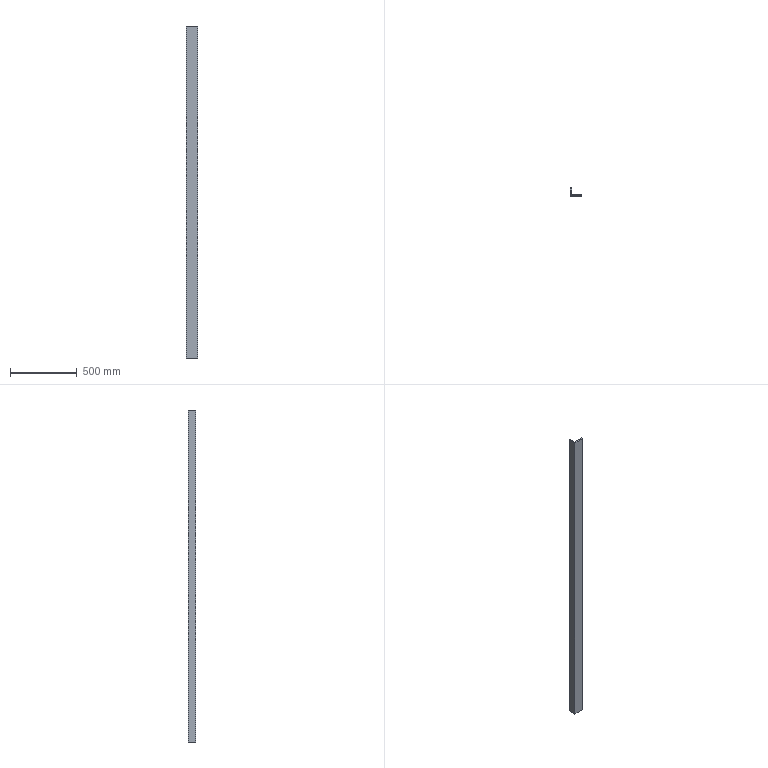Part | STEP file | Positioning angle steel_Default<As machined> | 1 solid | 8 faces | box 83 x 58 x 2484 mm | volume 2642976 mm3 | plane 8
STEP:
#1=CARTESIAN_POINT('',(0.,0.,0.));
#2=DIRECTION('',(0.,0.,1.));
#3=DIRECTION('',(1.,0.,0.));
#4=AXIS2_PLACEMENT_3D('',#1,#2,#3);
#5=CARTESIAN_POINT('',(2684.309,1399.529,5287.416));
#6=VERTEX_POINT('',#5);
#7=CARTESIAN_POINT('',(2684.309,1407.529,5287.416));
#8=VERTEX_POINT('',#7);
#9=CARTESIAN_POINT('',(2684.309,1399.529,5287.416));
#10=DIRECTION('',(0.,1.,0.));
#11=VECTOR('',#10,1.);
#12=LINE('',#9,#11);
#13=CARTESIAN_POINT('',(2684.309,1399.529,5388.673));
#14=DIRECTION('',(-1.,0.,0.));
#15=DIRECTION('',(0.,0.,1.));
#16=AXIS2_PLACEMENT_3D('',#13,#14,#15);
#17=PLANE('',#16);
#18=CARTESIAN_POINT('',(-101.257,0.));
#19=DIRECTION('',(0.,1.));
#20=VECTOR('',#19,1.);
#21=LINE('',#18,#20);
#22=(GEOMETRIC_REPRESENTATION_CONTEXT(2)PARAMETRIC_REPRESENTATION_CONTEXT()REPRESENTATION_CONTEXT('',''));
#23=DEFINITIONAL_REPRESENTATION('',(#21),#22);
#24=PCURVE('',#17,#23);
#25=CARTESIAN_POINT('',(1791.123,-1401.429,5287.416));
#26=DIRECTION('',(0.,0.,1.));
#27=DIRECTION('',(1.,0.,0.));
#28=AXIS2_PLACEMENT_3D('',#25,#26,#27);
#29=PLANE('',#28);
#30=CARTESIAN_POINT('',(893.186,2800.958));
#31=DIRECTION('',(0.,1.));
#32=VECTOR('',#31,1.);
#33=LINE('',#30,#32);
#34=(GEOMETRIC_REPRESENTATION_CONTEXT(2)PARAMETRIC_REPRESENTATION_CONTEXT()REPRESENTATION_CONTEXT('',''));
#35=DEFINITIONAL_REPRESENTATION('',(#33),#34);
#36=PCURVE('',#29,#35);
#37=SURFACE_CURVE('',#12,(#24,#36),.PCURVE_S1.);
#38=EDGE_CURVE('',#6,#8,#37,.T.);
#39=ORIENTED_EDGE('',*,*,#38,.F.);
#40=CARTESIAN_POINT('',(2684.309,1399.529,2803.416));
#41=VERTEX_POINT('',#40);
#42=CARTESIAN_POINT('',(2684.309,1399.529,5388.673));
#43=DIRECTION('',(0.,0.,-1.));
#44=VECTOR('',#43,1.);
#45=LINE('',#42,#44);
#46=CARTESIAN_POINT('',(0.,0.));
#47=DIRECTION('',(-1.,0.));
#48=VECTOR('',#47,1.);
#49=LINE('',#46,#48);
#50=(GEOMETRIC_REPRESENTATION_CONTEXT(2)PARAMETRIC_REPRESENTATION_CONTEXT()REPRESENTATION_CONTEXT('',''));
#51=DEFINITIONAL_REPRESENTATION('',(#49),#50);
#52=PCURVE('',#17,#51);
#53=CARTESIAN_POINT('',(2601.309,1399.529,5388.673));
#54=DIRECTION('',(0.,1.,0.));
#55=DIRECTION('',(0.,0.,1.));
#56=AXIS2_PLACEMENT_3D('',#53,#54,#55);
#57=PLANE('',#56);
#58=CARTESIAN_POINT('',(0.,83.));
#59=DIRECTION('',(-1.,0.));
#60=VECTOR('',#59,1.);
#61=LINE('',#58,#60);
#62=(GEOMETRIC_REPRESENTATION_CONTEXT(2)PARAMETRIC_REPRESENTATION_CONTEXT()REPRESENTATION_CONTEXT('',''));
#63=DEFINITIONAL_REPRESENTATION('',(#61),#62);
#64=PCURVE('',#57,#63);
#65=SURFACE_CURVE('',#45,(#52,#64),.PCURVE_S1.);
#66=EDGE_CURVE('',#6,#41,#65,.T.);
#67=ORIENTED_EDGE('',*,*,#66,.T.);
#68=CARTESIAN_POINT('',(2684.309,1407.529,2803.416));
#69=VERTEX_POINT('',#68);
#70=CARTESIAN_POINT('',(2684.309,1399.529,2803.416));
#71=DIRECTION('',(0.,1.,0.));
#72=VECTOR('',#71,1.);
#73=LINE('',#70,#72);
#74=CARTESIAN_POINT('',(-2585.257,0.));
#75=DIRECTION('',(0.,1.));
#76=VECTOR('',#75,1.);
#77=LINE('',#74,#76);
#78=(GEOMETRIC_REPRESENTATION_CONTEXT(2)PARAMETRIC_REPRESENTATION_CONTEXT()REPRESENTATION_CONTEXT('',''));
#79=DEFINITIONAL_REPRESENTATION('',(#77),#78);
#80=PCURVE('',#17,#79);
#81=CARTESIAN_POINT('',(0.,0.,2803.416));
#82=DIRECTION('',(0.,0.,1.));
#83=DIRECTION('',(1.,0.,0.));
#84=AXIS2_PLACEMENT_3D('',#81,#82,#83);
#85=PLANE('',#84);
#86=CARTESIAN_POINT('',(2684.309,1399.529));
#87=DIRECTION('',(0.,1.));
#88=VECTOR('',#87,1.);
#89=LINE('',#86,#88);
#90=(GEOMETRIC_REPRESENTATION_CONTEXT(2)PARAMETRIC_REPRESENTATION_CONTEXT()REPRESENTATION_CONTEXT('',''));
#91=DEFINITIONAL_REPRESENTATION('',(#89),#90);
#92=PCURVE('',#85,#91);
#93=SURFACE_CURVE('',#73,(#80,#92),.PCURVE_S1.);
#94=EDGE_CURVE('',#41,#69,#93,.T.);
#95=ORIENTED_EDGE('',*,*,#94,.T.);
#96=CARTESIAN_POINT('',(2684.309,1407.529,5388.673));
#97=DIRECTION('',(0.,0.,-1.));
#98=VECTOR('',#97,1.);
#99=LINE('',#96,#98);
#100=CARTESIAN_POINT('',(0.,8.));
#101=DIRECTION('',(-1.,0.));
#102=VECTOR('',#101,1.);
#103=LINE('',#100,#102);
#104=(GEOMETRIC_REPRESENTATION_CONTEXT(2)PARAMETRIC_REPRESENTATION_CONTEXT()REPRESENTATION_CONTEXT('',''));
#105=DEFINITIONAL_REPRESENTATION('',(#103),#104);
#106=PCURVE('',#17,#105);
#107=CARTESIAN_POINT('',(2684.309,1407.529,5388.673));
#108=DIRECTION('',(0.,-1.,0.));
#109=DIRECTION('',(0.,0.,-1.));
#110=AXIS2_PLACEMENT_3D('',#107,#108,#109);
#111=PLANE('',#110);
#112=CARTESIAN_POINT('',(0.,0.));
#113=DIRECTION('',(1.,0.));
#114=VECTOR('',#113,1.);
#115=LINE('',#112,#114);
#116=(GEOMETRIC_REPRESENTATION_CONTEXT(2)PARAMETRIC_REPRESENTATION_CONTEXT()REPRESENTATION_CONTEXT('',''));
#117=DEFINITIONAL_REPRESENTATION('',(#115),#116);
#118=PCURVE('',#111,#117);
#119=SURFACE_CURVE('',#99,(#106,#118),.PCURVE_S1.);
#120=EDGE_CURVE('',#8,#69,#119,.T.);
#121=ORIENTED_EDGE('',*,*,#120,.F.);
#122=EDGE_LOOP('',(#39,#67,#95,#121));
#123=FACE_BOUND('',#122,.T.);
#124=ADVANCED_FACE('',(#123),#17,.F.);
#125=CARTESIAN_POINT('',(2609.309,1407.529,5287.416));
#126=VERTEX_POINT('',#125);
#127=CARTESIAN_POINT('',(2684.309,1407.529,5287.416));
#128=DIRECTION('',(-1.,0.,0.));
#129=VECTOR('',#128,1.);
#130=LINE('',#127,#129);
#131=CARTESIAN_POINT('',(101.257,0.));
#132=DIRECTION('',(0.,-1.));
#133=VECTOR('',#132,1.);
#134=LINE('',#131,#133);
#135=(GEOMETRIC_REPRESENTATION_CONTEXT(2)PARAMETRIC_REPRESENTATION_CONTEXT()REPRESENTATION_CONTEXT('',''));
#136=DEFINITIONAL_REPRESENTATION('',(#134),#135);
#137=PCURVE('',#111,#136);
#138=CARTESIAN_POINT('',(893.186,2808.958));
#139=DIRECTION('',(-1.,0.));
#140=VECTOR('',#139,1.);
#141=LINE('',#138,#140);
#142=(GEOMETRIC_REPRESENTATION_CONTEXT(2)PARAMETRIC_REPRESENTATION_CONTEXT()REPRESENTATION_CONTEXT('',''));
#143=DEFINITIONAL_REPRESENTATION('',(#141),#142);
#144=PCURVE('',#29,#143);
#145=SURFACE_CURVE('',#130,(#137,#144),.PCURVE_S1.);
#146=EDGE_CURVE('',#8,#126,#145,.T.);
#147=ORIENTED_EDGE('',*,*,#146,.F.);
#148=ORIENTED_EDGE('',*,*,#120,.T.);
#149=CARTESIAN_POINT('',(2609.309,1407.529,2803.416));
#150=VERTEX_POINT('',#149);
#151=CARTESIAN_POINT('',(2684.309,1407.529,2803.416));
#152=DIRECTION('',(-1.,0.,0.));
#153=VECTOR('',#152,1.);
#154=LINE('',#151,#153);
#155=CARTESIAN_POINT('',(2585.257,0.));
#156=DIRECTION('',(0.,-1.));
#157=VECTOR('',#156,1.);
#158=LINE('',#155,#157);
#159=(GEOMETRIC_REPRESENTATION_CONTEXT(2)PARAMETRIC_REPRESENTATION_CONTEXT()REPRESENTATION_CONTEXT('',''));
#160=DEFINITIONAL_REPRESENTATION('',(#158),#159);
#161=PCURVE('',#111,#160);
#162=CARTESIAN_POINT('',(2684.309,1407.529));
#163=DIRECTION('',(-1.,0.));
#164=VECTOR('',#163,1.);
#165=LINE('',#162,#164);
#166=(GEOMETRIC_REPRESENTATION_CONTEXT(2)PARAMETRIC_REPRESENTATION_CONTEXT()REPRESENTATION_CONTEXT('',''));
#167=DEFINITIONAL_REPRESENTATION('',(#165),#166);
#168=PCURVE('',#85,#167);
#169=SURFACE_CURVE('',#154,(#161,#168),.PCURVE_S1.);
#170=EDGE_CURVE('',#69,#150,#169,.T.);
#171=ORIENTED_EDGE('',*,*,#170,.T.);
#172=CARTESIAN_POINT('',(2609.309,1407.529,5388.673));
#173=DIRECTION('',(0.,0.,-1.));
#174=VECTOR('',#173,1.);
#175=LINE('',#172,#174);
#176=CARTESIAN_POINT('',(0.,-75.));
#177=DIRECTION('',(1.,0.));
#178=VECTOR('',#177,1.);
#179=LINE('',#176,#178);
#180=(GEOMETRIC_REPRESENTATION_CONTEXT(2)PARAMETRIC_REPRESENTATION_CONTEXT()REPRESENTATION_CONTEXT('',''));
#181=DEFINITIONAL_REPRESENTATION('',(#179),#180);
#182=PCURVE('',#111,#181);
#183=CARTESIAN_POINT('',(2609.309,1407.529,5388.673));
#184=DIRECTION('',(-1.,0.,0.));
#185=DIRECTION('',(0.,0.,1.));
#186=AXIS2_PLACEMENT_3D('',#183,#184,#185);
#187=PLANE('',#186);
#188=CARTESIAN_POINT('',(0.,0.));
#189=DIRECTION('',(-1.,0.));
#190=VECTOR('',#189,1.);
#191=LINE('',#188,#190);
#192=(GEOMETRIC_REPRESENTATION_CONTEXT(2)PARAMETRIC_REPRESENTATION_CONTEXT()REPRESENTATION_CONTEXT('',''));
#193=DEFINITIONAL_REPRESENTATION('',(#191),#192);
#194=PCURVE('',#187,#193);
#195=SURFACE_CURVE('',#175,(#182,#194),.PCURVE_S1.);
#196=EDGE_CURVE('',#126,#150,#195,.T.);
#197=ORIENTED_EDGE('',*,*,#196,.F.);
#198=EDGE_LOOP('',(#147,#148,#171,#197));
#199=FACE_BOUND('',#198,.T.);
#200=ADVANCED_FACE('',(#199),#111,.F.);
#201=CARTESIAN_POINT('',(2609.309,1457.529,5287.416));
#202=VERTEX_POINT('',#201);
#203=CARTESIAN_POINT('',(2609.309,1407.529,5287.416));
#204=DIRECTION('',(0.,1.,0.));
#205=VECTOR('',#204,1.);
#206=LINE('',#203,#205);
#207=CARTESIAN_POINT('',(-101.257,0.));
#208=DIRECTION('',(0.,1.));
#209=VECTOR('',#208,1.);
#210=LINE('',#207,#209);
#211=(GEOMETRIC_REPRESENTATION_CONTEXT(2)PARAMETRIC_REPRESENTATION_CONTEXT()REPRESENTATION_CONTEXT('',''));
#212=DEFINITIONAL_REPRESENTATION('',(#210),#211);
#213=PCURVE('',#187,#212);
#214=CARTESIAN_POINT('',(818.186,2808.958));
#215=DIRECTION('',(0.,1.));
#216=VECTOR('',#215,1.);
#217=LINE('',#214,#216);
#218=(GEOMETRIC_REPRESENTATION_CONTEXT(2)PARAMETRIC_REPRESENTATION_CONTEXT()REPRESENTATION_CONTEXT('',''));
#219=DEFINITIONAL_REPRESENTATION('',(#217),#218);
#220=PCURVE('',#29,#219);
#221=SURFACE_CURVE('',#206,(#213,#220),.PCURVE_S1.);
#222=EDGE_CURVE('',#126,#202,#221,.T.);
#223=ORIENTED_EDGE('',*,*,#222,.F.);
#224=ORIENTED_EDGE('',*,*,#196,.T.);
#225=CARTESIAN_POINT('',(2609.309,1457.529,2803.416));
#226=VERTEX_POINT('',#225);
#227=CARTESIAN_POINT('',(2609.309,1407.529,2803.416));
#228=DIRECTION('',(0.,1.,0.));
#229=VECTOR('',#228,1.);
#230=LINE('',#227,#229);
#231=CARTESIAN_POINT('',(-2585.257,0.));
#232=DIRECTION('',(0.,1.));
#233=VECTOR('',#232,1.);
#234=LINE('',#231,#233);
#235=(GEOMETRIC_REPRESENTATION_CONTEXT(2)PARAMETRIC_REPRESENTATION_CONTEXT()REPRESENTATION_CONTEXT('',''));
#236=DEFINITIONAL_REPRESENTATION('',(#234),#235);
#237=PCURVE('',#187,#236);
#238=CARTESIAN_POINT('',(2609.309,1407.529));
#239=DIRECTION('',(0.,1.));
#240=VECTOR('',#239,1.);
#241=LINE('',#238,#240);
#242=(GEOMETRIC_REPRESENTATION_CONTEXT(2)PARAMETRIC_REPRESENTATION_CONTEXT()REPRESENTATION_CONTEXT('',''));
#243=DEFINITIONAL_REPRESENTATION('',(#241),#242);
#244=PCURVE('',#85,#243);
#245=SURFACE_CURVE('',#230,(#237,#244),.PCURVE_S1.);
#246=EDGE_CURVE('',#150,#226,#245,.T.);
#247=ORIENTED_EDGE('',*,*,#246,.T.);
#248=CARTESIAN_POINT('',(2609.309,1457.529,5388.673));
#249=DIRECTION('',(0.,0.,-1.));
#250=VECTOR('',#249,1.);
#251=LINE('',#248,#250);
#252=CARTESIAN_POINT('',(0.,50.));
#253=DIRECTION('',(-1.,0.));
#254=VECTOR('',#253,1.);
#255=LINE('',#252,#254);
#256=(GEOMETRIC_REPRESENTATION_CONTEXT(2)PARAMETRIC_REPRESENTATION_CONTEXT()REPRESENTATION_CONTEXT('',''));
#257=DEFINITIONAL_REPRESENTATION('',(#255),#256);
#258=PCURVE('',#187,#257);
#259=CARTESIAN_POINT('',(2609.309,1457.529,5388.673));
#260=DIRECTION('',(0.,-1.,0.));
#261=DIRECTION('',(0.,0.,-1.));
#262=AXIS2_PLACEMENT_3D('',#259,#260,#261);
#263=PLANE('',#262);
#264=CARTESIAN_POINT('',(0.,0.));
#265=DIRECTION('',(1.,0.));
#266=VECTOR('',#265,1.);
#267=LINE('',#264,#266);
#268=(GEOMETRIC_REPRESENTATION_CONTEXT(2)PARAMETRIC_REPRESENTATION_CONTEXT()REPRESENTATION_CONTEXT('',''));
#269=DEFINITIONAL_REPRESENTATION('',(#267),#268);
#270=PCURVE('',#263,#269);
#271=SURFACE_CURVE('',#251,(#258,#270),.PCURVE_S1.);
#272=EDGE_CURVE('',#202,#226,#271,.T.);
#273=ORIENTED_EDGE('',*,*,#272,.F.);
#274=EDGE_LOOP('',(#223,#224,#247,#273));
#275=FACE_BOUND('',#274,.T.);
#276=ADVANCED_FACE('',(#275),#187,.F.);
#277=CARTESIAN_POINT('',(2601.309,1457.529,5287.416));
#278=VERTEX_POINT('',#277);
#279=CARTESIAN_POINT('',(2609.309,1457.529,5287.416));
#280=DIRECTION('',(-1.,0.,0.));
#281=VECTOR('',#280,1.);
#282=LINE('',#279,#281);
#283=CARTESIAN_POINT('',(101.257,0.));
#284=DIRECTION('',(0.,-1.));
#285=VECTOR('',#284,1.);
#286=LINE('',#283,#285);
#287=(GEOMETRIC_REPRESENTATION_CONTEXT(2)PARAMETRIC_REPRESENTATION_CONTEXT()REPRESENTATION_CONTEXT('',''));
#288=DEFINITIONAL_REPRESENTATION('',(#286),#287);
#289=PCURVE('',#263,#288);
#290=CARTESIAN_POINT('',(818.186,2858.958));
#291=DIRECTION('',(-1.,0.));
#292=VECTOR('',#291,1.);
#293=LINE('',#290,#292);
#294=(GEOMETRIC_REPRESENTATION_CONTEXT(2)PARAMETRIC_REPRESENTATION_CONTEXT()REPRESENTATION_CONTEXT('',''));
#295=DEFINITIONAL_REPRESENTATION('',(#293),#294);
#296=PCURVE('',#29,#295);
#297=SURFACE_CURVE('',#282,(#289,#296),.PCURVE_S1.);
#298=EDGE_CURVE('',#202,#278,#297,.T.);
#299=ORIENTED_EDGE('',*,*,#298,.F.);
#300=ORIENTED_EDGE('',*,*,#272,.T.);
#301=CARTESIAN_POINT('',(2601.309,1457.529,2803.416));
#302=VERTEX_POINT('',#301);
#303=CARTESIAN_POINT('',(2609.309,1457.529,2803.416));
#304=DIRECTION('',(-1.,0.,0.));
#305=VECTOR('',#304,1.);
#306=LINE('',#303,#305);
#307=CARTESIAN_POINT('',(2585.257,0.));
#308=DIRECTION('',(0.,-1.));
#309=VECTOR('',#308,1.);
#310=LINE('',#307,#309);
#311=(GEOMETRIC_REPRESENTATION_CONTEXT(2)PARAMETRIC_REPRESENTATION_CONTEXT()REPRESENTATION_CONTEXT('',''));
#312=DEFINITIONAL_REPRESENTATION('',(#310),#311);
#313=PCURVE('',#263,#312);
#314=CARTESIAN_POINT('',(2609.309,1457.529));
#315=DIRECTION('',(-1.,0.));
#316=VECTOR('',#315,1.);
#317=LINE('',#314,#316);
#318=(GEOMETRIC_REPRESENTATION_CONTEXT(2)PARAMETRIC_REPRESENTATION_CONTEXT()REPRESENTATION_CONTEXT('',''));
#319=DEFINITIONAL_REPRESENTATION('',(#317),#318);
#320=PCURVE('',#85,#319);
#321=SURFACE_CURVE('',#306,(#313,#320),.PCURVE_S1.);
#322=EDGE_CURVE('',#226,#302,#321,.T.);
#323=ORIENTED_EDGE('',*,*,#322,.T.);
#324=CARTESIAN_POINT('',(2601.309,1457.529,5388.673));
#325=DIRECTION('',(0.,0.,-1.));
#326=VECTOR('',#325,1.);
#327=LINE('',#324,#326);
#328=CARTESIAN_POINT('',(0.,-8.));
#329=DIRECTION('',(1.,0.));
#330=VECTOR('',#329,1.);
#331=LINE('',#328,#330);
#332=(GEOMETRIC_REPRESENTATION_CONTEXT(2)PARAMETRIC_REPRESENTATION_CONTEXT()REPRESENTATION_CONTEXT('',''));
#333=DEFINITIONAL_REPRESENTATION('',(#331),#332);
#334=PCURVE('',#263,#333);
#335=CARTESIAN_POINT('',(2601.309,1457.529,5388.673));
#336=DIRECTION('',(1.,0.,0.));
#337=DIRECTION('',(0.,0.,-1.));
#338=AXIS2_PLACEMENT_3D('',#335,#336,#337);
#339=PLANE('',#338);
#340=CARTESIAN_POINT('',(0.,0.));
#341=DIRECTION('',(1.,0.));
#342=VECTOR('',#341,1.);
#343=LINE('',#340,#342);
#344=(GEOMETRIC_REPRESENTATION_CONTEXT(2)PARAMETRIC_REPRESENTATION_CONTEXT()REPRESENTATION_CONTEXT('',''));
#345=DEFINITIONAL_REPRESENTATION('',(#343),#344);
#346=PCURVE('',#339,#345);
#347=SURFACE_CURVE('',#327,(#334,#346),.PCURVE_S1.);
#348=EDGE_CURVE('',#278,#302,#347,.T.);
#349=ORIENTED_EDGE('',*,*,#348,.F.);
#350=EDGE_LOOP('',(#299,#300,#323,#349));
#351=FACE_BOUND('',#350,.T.);
#352=ADVANCED_FACE('',(#351),#263,.F.);
#353=CARTESIAN_POINT('',(2601.309,1399.529,5287.416));
#354=VERTEX_POINT('',#353);
#355=CARTESIAN_POINT('',(2601.309,1457.529,5287.416));
#356=DIRECTION('',(0.,-1.,0.));
#357=VECTOR('',#356,1.);
#358=LINE('',#355,#357);
#359=CARTESIAN_POINT('',(101.257,0.));
#360=DIRECTION('',(0.,-1.));
#361=VECTOR('',#360,1.);
#362=LINE('',#359,#361);
#363=(GEOMETRIC_REPRESENTATION_CONTEXT(2)PARAMETRIC_REPRESENTATION_CONTEXT()REPRESENTATION_CONTEXT('',''));
#364=DEFINITIONAL_REPRESENTATION('',(#362),#363);
#365=PCURVE('',#339,#364);
#366=CARTESIAN_POINT('',(810.186,2858.958));
#367=DIRECTION('',(0.,-1.));
#368=VECTOR('',#367,1.);
#369=LINE('',#366,#368);
#370=(GEOMETRIC_REPRESENTATION_CONTEXT(2)PARAMETRIC_REPRESENTATION_CONTEXT()REPRESENTATION_CONTEXT('',''));
#371=DEFINITIONAL_REPRESENTATION('',(#369),#370);
#372=PCURVE('',#29,#371);
#373=SURFACE_CURVE('',#358,(#365,#372),.PCURVE_S1.);
#374=EDGE_CURVE('',#278,#354,#373,.T.);
#375=ORIENTED_EDGE('',*,*,#374,.F.);
#376=ORIENTED_EDGE('',*,*,#348,.T.);
#377=CARTESIAN_POINT('',(2601.309,1399.529,2803.416));
#378=VERTEX_POINT('',#377);
#379=CARTESIAN_POINT('',(2601.309,1457.529,2803.416));
#380=DIRECTION('',(0.,-1.,0.));
#381=VECTOR('',#380,1.);
#382=LINE('',#379,#381);
#383=CARTESIAN_POINT('',(2585.257,0.));
#384=DIRECTION('',(0.,-1.));
#385=VECTOR('',#384,1.);
#386=LINE('',#383,#385);
#387=(GEOMETRIC_REPRESENTATION_CONTEXT(2)PARAMETRIC_REPRESENTATION_CONTEXT()REPRESENTATION_CONTEXT('',''));
#388=DEFINITIONAL_REPRESENTATION('',(#386),#387);
#389=PCURVE('',#339,#388);
#390=CARTESIAN_POINT('',(2601.309,1457.529));
#391=DIRECTION('',(0.,-1.));
#392=VECTOR('',#391,1.);
#393=LINE('',#390,#392);
#394=(GEOMETRIC_REPRESENTATION_CONTEXT(2)PARAMETRIC_REPRESENTATION_CONTEXT()REPRESENTATION_CONTEXT('',''));
#395=DEFINITIONAL_REPRESENTATION('',(#393),#394);
#396=PCURVE('',#85,#395);
#397=SURFACE_CURVE('',#382,(#389,#396),.PCURVE_S1.);
#398=EDGE_CURVE('',#302,#378,#397,.T.);
#399=ORIENTED_EDGE('',*,*,#398,.T.);
#400=CARTESIAN_POINT('',(2601.309,1399.529,5388.673));
#401=DIRECTION('',(0.,0.,-1.));
#402=VECTOR('',#401,1.);
#403=LINE('',#400,#402);
#404=CARTESIAN_POINT('',(0.,-58.));
#405=DIRECTION('',(1.,0.));
#406=VECTOR('',#405,1.);
#407=LINE('',#404,#406);
#408=(GEOMETRIC_REPRESENTATION_CONTEXT(2)PARAMETRIC_REPRESENTATION_CONTEXT()REPRESENTATION_CONTEXT('',''));
#409=DEFINITIONAL_REPRESENTATION('',(#407),#408);
#410=PCURVE('',#339,#409);
#411=CARTESIAN_POINT('',(0.,0.));
#412=DIRECTION('',(-1.,0.));
#413=VECTOR('',#412,1.);
#414=LINE('',#411,#413);
#415=(GEOMETRIC_REPRESENTATION_CONTEXT(2)PARAMETRIC_REPRESENTATION_CONTEXT()REPRESENTATION_CONTEXT('',''));
#416=DEFINITIONAL_REPRESENTATION('',(#414),#415);
#417=PCURVE('',#57,#416);
#418=SURFACE_CURVE('',#403,(#410,#417),.PCURVE_S1.);
#419=EDGE_CURVE('',#354,#378,#418,.T.);
#420=ORIENTED_EDGE('',*,*,#419,.F.);
#421=EDGE_LOOP('',(#375,#376,#399,#420));
#422=FACE_BOUND('',#421,.T.);
#423=ADVANCED_FACE('',(#422),#339,.F.);
#424=CARTESIAN_POINT('',(2601.309,1399.529,5287.416));
#425=DIRECTION('',(1.,0.,0.));
#426=VECTOR('',#425,1.);
#427=LINE('',#424,#426);
#428=CARTESIAN_POINT('',(-101.257,0.));
#429=DIRECTION('',(0.,1.));
#430=VECTOR('',#429,1.);
#431=LINE('',#428,#430);
#432=(GEOMETRIC_REPRESENTATION_CONTEXT(2)PARAMETRIC_REPRESENTATION_CONTEXT()REPRESENTATION_CONTEXT('',''));
#433=DEFINITIONAL_REPRESENTATION('',(#431),#432);
#434=PCURVE('',#57,#433);
#435=CARTESIAN_POINT('',(810.186,2800.958));
#436=DIRECTION('',(1.,0.));
#437=VECTOR('',#436,1.);
#438=LINE('',#435,#437);
#439=(GEOMETRIC_REPRESENTATION_CONTEXT(2)PARAMETRIC_REPRESENTATION_CONTEXT()REPRESENTATION_CONTEXT('',''));
#440=DEFINITIONAL_REPRESENTATION('',(#438),#439);
#441=PCURVE('',#29,#440);
#442=SURFACE_CURVE('',#427,(#434,#441),.PCURVE_S1.);
#443=EDGE_CURVE('',#354,#6,#442,.T.);
#444=ORIENTED_EDGE('',*,*,#443,.F.);
#445=ORIENTED_EDGE('',*,*,#419,.T.);
#446=CARTESIAN_POINT('',(2601.309,1399.529,2803.416));
#447=DIRECTION('',(1.,0.,0.));
#448=VECTOR('',#447,1.);
#449=LINE('',#446,#448);
#450=CARTESIAN_POINT('',(-2585.257,0.));
#451=DIRECTION('',(0.,1.));
#452=VECTOR('',#451,1.);
#453=LINE('',#450,#452);
#454=(GEOMETRIC_REPRESENTATION_CONTEXT(2)PARAMETRIC_REPRESENTATION_CONTEXT()REPRESENTATION_CONTEXT('',''));
#455=DEFINITIONAL_REPRESENTATION('',(#453),#454);
#456=PCURVE('',#57,#455);
#457=CARTESIAN_POINT('',(2601.309,1399.529));
#458=DIRECTION('',(1.,0.));
#459=VECTOR('',#458,1.);
#460=LINE('',#457,#459);
#461=(GEOMETRIC_REPRESENTATION_CONTEXT(2)PARAMETRIC_REPRESENTATION_CONTEXT()REPRESENTATION_CONTEXT('',''));
#462=DEFINITIONAL_REPRESENTATION('',(#460),#461);
#463=PCURVE('',#85,#462);
#464=SURFACE_CURVE('',#449,(#456,#463),.PCURVE_S1.);
#465=EDGE_CURVE('',#378,#41,#464,.T.);
#466=ORIENTED_EDGE('',*,*,#465,.T.);
#467=ORIENTED_EDGE('',*,*,#66,.F.);
#468=EDGE_LOOP('',(#444,#445,#466,#467));
#469=FACE_BOUND('',#468,.T.);
#470=ADVANCED_FACE('',(#469),#57,.F.);
#471=ORIENTED_EDGE('',*,*,#94,.F.);
#472=ORIENTED_EDGE('',*,*,#465,.F.);
#473=ORIENTED_EDGE('',*,*,#398,.F.);
#474=ORIENTED_EDGE('',*,*,#322,.F.);
#475=ORIENTED_EDGE('',*,*,#246,.F.);
#476=ORIENTED_EDGE('',*,*,#170,.F.);
#477=EDGE_LOOP('',(#471,#472,#473,#474,#475,#476));
#478=FACE_BOUND('',#477,.T.);
#479=ADVANCED_FACE('',(#478),#85,.F.);
#480=ORIENTED_EDGE('',*,*,#443,.T.);
#481=ORIENTED_EDGE('',*,*,#38,.T.);
#482=ORIENTED_EDGE('',*,*,#146,.T.);
#483=ORIENTED_EDGE('',*,*,#222,.T.);
#484=ORIENTED_EDGE('',*,*,#298,.T.);
#485=ORIENTED_EDGE('',*,*,#374,.T.);
#486=EDGE_LOOP('',(#480,#481,#482,#483,#484,#485));
#487=FACE_BOUND('',#486,.T.);
#488=ADVANCED_FACE('',(#487),#29,.T.);
#489=CLOSED_SHELL('',(#124,#200,#276,#352,#423,#470,#479,#488));
#490=MANIFOLD_SOLID_BREP('',#489);
#491=(LENGTH_UNIT()NAMED_UNIT(*)SI_UNIT(.MILLI.,.METRE.));
#492=UNCERTAINTY_MEASURE_WITH_UNIT(LENGTH_MEASURE(0.0000001),#491,'','');
#493=(NAMED_UNIT(*)PLANE_ANGLE_UNIT()SI_UNIT($,.RADIAN.));
#494=(NAMED_UNIT(*)SI_UNIT($,.STERADIAN.)SOLID_ANGLE_UNIT());
#495=(GEOMETRIC_REPRESENTATION_CONTEXT(3)GLOBAL_UNCERTAINTY_ASSIGNED_CONTEXT((#492))GLOBAL_UNIT_ASSIGNED_CONTEXT((#491,#493,#494))REPRESENTATION_CONTEXT('',''));
#496=ADVANCED_BREP_SHAPE_REPRESENTATION('',(#4,#490),#495);